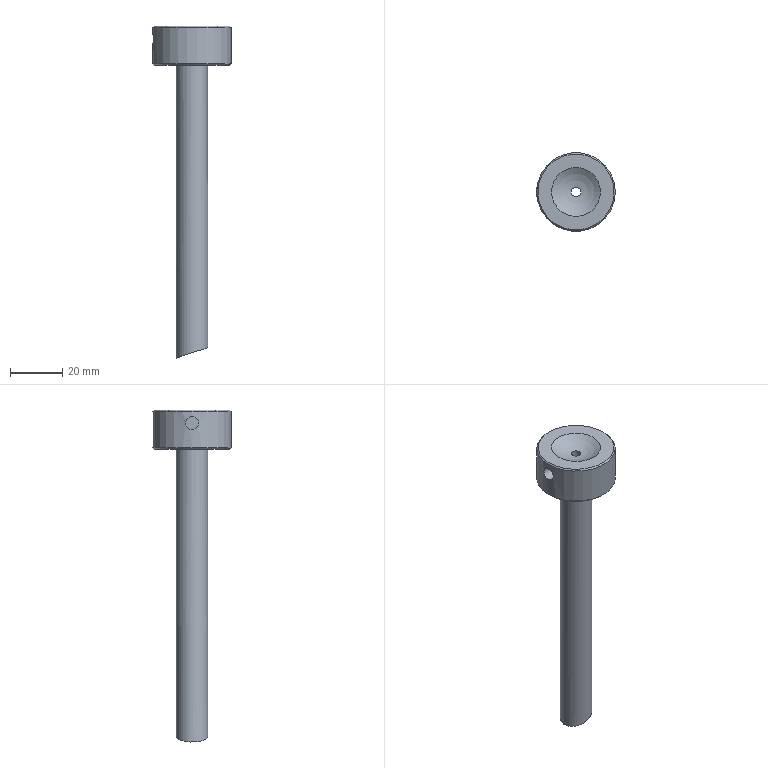Part | NX | features solid 2 | 1 solid | 11 faces | box 30 x 30 x 126.717 mm | volume 19254 mm3 | plane 3 | cylinder 3 | cone 3 | spline 1 | sphere 1 | commonest cylinder face diameters 5 x1 12 x1 30 x1
STEP:
#1=CARTESIAN_POINT('',(9.327,0.,140.5));
#2=VERTEX_POINT('',#1);
#3=CARTESIAN_POINT('',(0.,0.,140.5));
#4=DIRECTION('',(0.,0.,1.));
#5=DIRECTION('',(1.,0.,0.));
#6=AXIS2_PLACEMENT_3D('',#3,#4,#5);
#7=CIRCLE('',#6,9.327);
#8=EDGE_CURVE('',#2,#2,#7,.T.);
#9=ORIENTED_EDGE('',*,*,#8,.F.);
#10=EDGE_LOOP('',(#9));
#11=FACE_BOUND('',#10,.T.);
#12=CARTESIAN_POINT('',(14.5,0.,140.5));
#13=VERTEX_POINT('',#12);
#14=CARTESIAN_POINT('',(0.,0.,140.5));
#15=DIRECTION('',(0.,0.,1.));
#16=DIRECTION('',(1.,0.,0.));
#17=AXIS2_PLACEMENT_3D('',#14,#15,#16);
#18=CIRCLE('',#17,14.5);
#19=EDGE_CURVE('',#13,#13,#18,.T.);
#20=ORIENTED_EDGE('',*,*,#19,.T.);
#21=EDGE_LOOP('',(#20));
#22=FACE_BOUND('',#21,.T.);
#23=CARTESIAN_POINT('',(0.,0.,140.5));
#24=DIRECTION('',(0.,0.,1.));
#25=DIRECTION('',(1.,0.,0.));
#26=AXIS2_PLACEMENT_3D('',#23,#24,#25);
#27=PLANE('',#26);
#28=ADVANCED_FACE('',(#11,#22),#27,.T.);
#29=CARTESIAN_POINT('',(-6.,0.,125.5));
#30=VERTEX_POINT('',#29);
#31=CARTESIAN_POINT('',(0.,0.,125.5));
#32=DIRECTION('',(0.,0.,-1.));
#33=DIRECTION('',(-1.,0.,0.));
#34=AXIS2_PLACEMENT_3D('',#31,#32,#33);
#35=CIRCLE('',#34,6.);
#36=EDGE_CURVE('',#30,#30,#35,.T.);
#37=ORIENTED_EDGE('',*,*,#36,.F.);
#38=EDGE_LOOP('',(#37));
#39=FACE_BOUND('',#38,.T.);
#40=CARTESIAN_POINT('',(-14.5,0.,125.5));
#41=VERTEX_POINT('',#40);
#42=CARTESIAN_POINT('',(0.,0.,125.5));
#43=DIRECTION('',(0.,0.,-1.));
#44=DIRECTION('',(-1.,0.,0.));
#45=AXIS2_PLACEMENT_3D('',#42,#43,#44);
#46=CIRCLE('',#45,14.5);
#47=EDGE_CURVE('',#41,#41,#46,.T.);
#48=ORIENTED_EDGE('',*,*,#47,.T.);
#49=EDGE_LOOP('',(#48));
#50=FACE_BOUND('',#49,.T.);
#51=CARTESIAN_POINT('',(0.,0.,125.5));
#52=DIRECTION('',(0.,0.,-1.));
#53=DIRECTION('',(-1.,0.,0.));
#54=AXIS2_PLACEMENT_3D('',#51,#52,#53);
#55=PLANE('',#54);
#56=ADVANCED_FACE('',(#39,#50),#55,.T.);
#57=CARTESIAN_POINT('',(-15.,0.,138.));
#58=VERTEX_POINT('',#57);
#59=CARTESIAN_POINT('',(-14.896,-1.961,137.457));
#60=CARTESIAN_POINT('',(-15.052,0.0004642,138.271));
#61=CARTESIAN_POINT('',(-14.896,1.959,137.458));
#62=CARTESIAN_POINT('',(-14.737,2.77,135.502));
#63=CARTESIAN_POINT('',(-14.896,1.96,133.541));
#64=CARTESIAN_POINT('',(-15.052,0.0007333,132.73));
#65=CARTESIAN_POINT('',(-14.896,-1.957,133.539));
#66=CARTESIAN_POINT('',(-14.737,-2.771,135.498));
#67=CARTESIAN_POINT('',(-14.896,-1.961,137.457));
#68=CARTESIAN_POINT('',(-15.052,0.0004642,138.271));
#69=CARTESIAN_POINT('',(-14.896,1.959,137.458));
#70=B_SPLINE_CURVE_WITH_KNOTS('',3,(#59,#60,#61,#62,#63,#64,#65,#66,#67,#68,#69),.UNSPECIFIED.,.T.,.F.,(1,1,1,1,1,1,1,1,1,1,1,1,1,1,1),(-0.005872,-0.003914,-0.001957,0.,0.001957,0.003914,0.005872,0.007829,0.009786,0.01174,0.0137,0.01566,0.01761,0.01957,0.02153),.UNSPECIFIED.);
#71=EDGE_CURVE('',#58,#58,#70,.T.);
#72=ORIENTED_EDGE('',*,*,#71,.F.);
#73=EDGE_LOOP('',(#72));
#74=FACE_BOUND('',#73,.T.);
#75=CARTESIAN_POINT('',(-15.,0.,126.));
#76=VERTEX_POINT('',#75);
#77=CARTESIAN_POINT('',(0.,0.,126.));
#78=DIRECTION('',(0.,0.,-1.));
#79=DIRECTION('',(-1.,0.,0.));
#80=AXIS2_PLACEMENT_3D('',#77,#78,#79);
#81=CIRCLE('',#80,15.);
#82=EDGE_CURVE('',#76,#76,#81,.F.);
#83=ORIENTED_EDGE('',*,*,#82,.T.);
#84=EDGE_LOOP('',(#83));
#85=FACE_BOUND('',#84,.T.);
#86=CARTESIAN_POINT('',(15.,0.,140.));
#87=VERTEX_POINT('',#86);
#88=CARTESIAN_POINT('',(0.,0.,140.));
#89=DIRECTION('',(0.,0.,1.));
#90=DIRECTION('',(1.,0.,0.));
#91=AXIS2_PLACEMENT_3D('',#88,#89,#90);
#92=CIRCLE('',#91,15.);
#93=EDGE_CURVE('',#87,#87,#92,.F.);
#94=ORIENTED_EDGE('',*,*,#93,.T.);
#95=EDGE_LOOP('',(#94));
#96=FACE_BOUND('',#95,.T.);
#97=CARTESIAN_POINT('',(0.,0.,125.5));
#98=DIRECTION('',(0.,0.,1.));
#99=DIRECTION('',(1.,0.,0.));
#100=AXIS2_PLACEMENT_3D('',#97,#98,#99);
#101=CYLINDRICAL_SURFACE('',#100,15.);
#102=ADVANCED_FACE('',(#74,#85,#96),#101,.T.);
#103=ORIENTED_EDGE('',*,*,#47,.F.);
#104=EDGE_LOOP('',(#103));
#105=FACE_BOUND('',#104,.T.);
#106=ORIENTED_EDGE('',*,*,#82,.F.);
#107=EDGE_LOOP('',(#106));
#108=FACE_BOUND('',#107,.T.);
#109=CARTESIAN_POINT('',(0.,0.,126.));
#110=DIRECTION('',(0.,0.,1.));
#111=DIRECTION('',(1.,0.,0.));
#112=AXIS2_PLACEMENT_3D('',#109,#110,#111);
#113=CONICAL_SURFACE('',#112,15.,0.7854);
#114=ADVANCED_FACE('',(#105,#108),#113,.T.);
#115=ORIENTED_EDGE('',*,*,#19,.F.);
#116=EDGE_LOOP('',(#115));
#117=FACE_BOUND('',#116,.T.);
#118=ORIENTED_EDGE('',*,*,#93,.F.);
#119=EDGE_LOOP('',(#118));
#120=FACE_BOUND('',#119,.T.);
#121=CARTESIAN_POINT('',(0.,0.,140.));
#122=DIRECTION('',(0.,0.,-1.));
#123=DIRECTION('',(-1.,0.,0.));
#124=AXIS2_PLACEMENT_3D('',#121,#122,#123);
#125=CONICAL_SURFACE('',#124,15.,0.7854);
#126=ADVANCED_FACE('',(#117,#120),#125,.T.);
#127=CARTESIAN_POINT('',(-3.104,2.346,14.831));
#128=VERTEX_POINT('',#127);
#129=CARTESIAN_POINT('',(-4.293,-0.6648,14.409));
#130=CARTESIAN_POINT('',(-3.424,2.631,14.724));
#131=CARTESIAN_POINT('',(-0.6353,4.217,15.682));
#132=CARTESIAN_POINT('',(2.463,3.492,16.658));
#133=CARTESIAN_POINT('',(4.249,0.663,17.182));
#134=CARTESIAN_POINT('',(3.386,-2.632,16.932));
#135=CARTESIAN_POINT('',(0.5623,-4.224,16.069));
#136=CARTESIAN_POINT('',(-2.512,-3.48,15.046));
#137=CARTESIAN_POINT('',(-4.293,-0.6648,14.409));
#138=CARTESIAN_POINT('',(-3.424,2.631,14.724));
#139=CARTESIAN_POINT('',(-0.6353,4.217,15.682));
#140=B_SPLINE_CURVE_WITH_KNOTS('',3,(#129,#130,#131,#132,#133,#134,#135,#136,#137,#138,#139),.UNSPECIFIED.,.T.,.F.,(1,1,1,1,1,1,1,1,1,1,1,1,1,1,1),(-0.009313,-0.006208,-0.003104,0.,0.003104,0.006208,0.009313,0.01242,0.01552,0.01863,0.02173,0.02483,0.02794,0.03104,0.03415),.UNSPECIFIED.);
#141=EDGE_CURVE('',#128,#128,#140,.T.);
#142=ORIENTED_EDGE('',*,*,#141,.F.);
#143=EDGE_LOOP('',(#142));
#144=FACE_BOUND('',#143,.T.);
#145=CARTESIAN_POINT('',(-5.973,0.5729,13.792));
#146=VERTEX_POINT('',#145);
#147=CARTESIAN_POINT('',(-4.144,5.179,14.485));
#148=CARTESIAN_POINT('',(-6.663,0.6502,13.528));
#149=CARTESIAN_POINT('',(-5.039,-4.342,14.153));
#150=CARTESIAN_POINT('',(-0.6317,-6.572,15.703));
#151=CARTESIAN_POINT('',(4.133,-5.207,17.166));
#152=CARTESIAN_POINT('',(6.662,-0.6502,17.866));
#153=CARTESIAN_POINT('',(5.051,4.35,17.426));
#154=CARTESIAN_POINT('',(0.5479,6.585,16.084));
#155=CARTESIAN_POINT('',(-4.144,5.179,14.485));
#156=CARTESIAN_POINT('',(-6.663,0.6502,13.528));
#157=CARTESIAN_POINT('',(-5.039,-4.342,14.153));
#158=B_SPLINE_CURVE_WITH_KNOTS('',3,(#147,#148,#149,#150,#151,#152,#153,#154,#155,#156,#157),.UNSPECIFIED.,.T.,.F.,(1,1,1,1,1,1,1,1,1,1,1,1,1,1,1),(-0.01444,-0.009626,-0.004813,0.,0.004813,0.009626,0.01444,0.01925,0.02407,0.02888,0.03369,0.0385,0.04332,0.04813,0.05294),.UNSPECIFIED.);
#159=EDGE_CURVE('',#146,#146,#158,.T.);
#160=ORIENTED_EDGE('',*,*,#159,.F.);
#161=EDGE_LOOP('',(#160));
#162=FACE_BOUND('',#161,.T.);
#163=CARTESIAN_POINT('',(-6.105,6.11,13.742));
#164=CARTESIAN_POINT('',(-6.105,-6.095,13.742));
#165=CARTESIAN_POINT('',(-2.088,6.11,15.255));
#166=CARTESIAN_POINT('',(-2.088,-6.095,15.255));
#167=CARTESIAN_POINT('',(1.987,6.11,16.562));
#168=CARTESIAN_POINT('',(1.987,-6.095,16.562));
#169=CARTESIAN_POINT('',(6.109,6.11,17.714));
#170=CARTESIAN_POINT('',(6.109,-6.095,17.714));
#171=B_SPLINE_SURFACE_WITH_KNOTS('',3,1,((#163,#164),(#165,#166),(#167,#168),(#169,#170)),.SURF_OF_LINEAR_EXTRUSION.,.F.,.F.,.F.,(4,4),(2,2),(0.6579,0.7302),(0.,1.),.PIECEWISE_BEZIER_KNOTS.);
#172=ADVANCED_FACE('',(#144,#162),#171,.T.);
#173=ORIENTED_EDGE('',*,*,#159,.T.);
#174=EDGE_LOOP('',(#173));
#175=FACE_BOUND('',#174,.T.);
#176=ORIENTED_EDGE('',*,*,#36,.T.);
#177=EDGE_LOOP('',(#176));
#178=FACE_BOUND('',#177,.T.);
#179=CARTESIAN_POINT('',(0.,0.,125.5));
#180=DIRECTION('',(0.,0.,-1.));
#181=DIRECTION('',(1.,0.,0.));
#182=AXIS2_PLACEMENT_3D('',#179,#180,#181);
#183=CYLINDRICAL_SURFACE('',#182,6.);
#184=ADVANCED_FACE('',(#175,#178),#183,.T.);
#185=CARTESIAN_POINT('',(1.748,0.,137.596));
#186=VERTEX_POINT('',#185);
#187=CARTESIAN_POINT('',(0.,0.,137.596));
#188=DIRECTION('',(0.,0.,1.));
#189=DIRECTION('',(1.,0.,0.));
#190=AXIS2_PLACEMENT_3D('',#187,#188,#189);
#191=CIRCLE('',#190,1.748);
#192=EDGE_CURVE('',#186,#186,#191,.T.);
#193=ORIENTED_EDGE('',*,*,#192,.T.);
#194=EDGE_LOOP('',(#193));
#195=FACE_BOUND('',#194,.T.);
#196=ORIENTED_EDGE('',*,*,#141,.T.);
#197=EDGE_LOOP('',(#196));
#198=FACE_BOUND('',#197,.T.);
#199=CARTESIAN_POINT('',(0.,0.,137.5));
#200=DIRECTION('',(0.,0.,-1.));
#201=DIRECTION('',(1.,0.,0.));
#202=AXIS2_PLACEMENT_3D('',#199,#200,#201);
#203=CONICAL_SURFACE('',#202,1.75,0.01745);
#204=ADVANCED_FACE('',(#195,#198),#203,.F.);
#205=ORIENTED_EDGE('',*,*,#8,.T.);
#206=EDGE_LOOP('',(#205));
#207=FACE_BOUND('',#206,.T.);
#208=ORIENTED_EDGE('',*,*,#192,.F.);
#209=EDGE_LOOP('',(#208));
#210=FACE_BOUND('',#209,.T.);
#211=CARTESIAN_POINT('',(0.,0.,153.5));
#212=DIRECTION('',(0.,0.,1.));
#213=DIRECTION('',(1.,0.,0.));
#214=AXIS2_PLACEMENT_3D('',#211,#212,#213);
#215=SPHERICAL_SURFACE('',#214,16.);
#216=ADVANCED_FACE('',(#207,#210),#215,.F.);
#217=CARTESIAN_POINT('',(-8.,0.,138.));
#218=VERTEX_POINT('',#217);
#219=CARTESIAN_POINT('',(-8.,0.,135.5));
#220=DIRECTION('',(-1.,0.,0.));
#221=DIRECTION('',(0.,0.,1.));
#222=AXIS2_PLACEMENT_3D('',#219,#220,#221);
#223=CIRCLE('',#222,2.5);
#224=EDGE_CURVE('',#218,#218,#223,.F.);
#225=ORIENTED_EDGE('',*,*,#224,.F.);
#226=EDGE_LOOP('',(#225));
#227=FACE_BOUND('',#226,.T.);
#228=CARTESIAN_POINT('',(-8.,0.,135.5));
#229=DIRECTION('',(1.,0.,0.));
#230=DIRECTION('',(0.,1.,0.));
#231=AXIS2_PLACEMENT_3D('',#228,#229,#230);
#232=PLANE('',#231);
#233=ADVANCED_FACE('',(#227),#232,.F.);
#234=ORIENTED_EDGE('',*,*,#71,.T.);
#235=EDGE_LOOP('',(#234));
#236=FACE_BOUND('',#235,.T.);
#237=ORIENTED_EDGE('',*,*,#224,.T.);
#238=EDGE_LOOP('',(#237));
#239=FACE_BOUND('',#238,.T.);
#240=CARTESIAN_POINT('',(-8.,0.,135.5));
#241=DIRECTION('',(-1.,0.,0.));
#242=DIRECTION('',(0.,0.,1.));
#243=AXIS2_PLACEMENT_3D('',#240,#241,#242);
#244=CYLINDRICAL_SURFACE('',#243,2.5);
#245=ADVANCED_FACE('',(#236,#239),#244,.F.);
#246=CLOSED_SHELL('',(#28,#56,#102,#114,#126,#172,#184,#204,#216,#233,#245));
#247=MANIFOLD_SOLID_BREP('',#246);
#248=(LENGTH_UNIT()NAMED_UNIT(*)SI_UNIT(.MILLI.,.METRE.));
#249=UNCERTAINTY_MEASURE_WITH_UNIT(LENGTH_MEASURE(0.0508),#248,'','');
#250=(NAMED_UNIT(*)PLANE_ANGLE_UNIT()SI_UNIT($,.RADIAN.));
#251=(NAMED_UNIT(*)SI_UNIT($,.STERADIAN.)SOLID_ANGLE_UNIT());
#252=(GEOMETRIC_REPRESENTATION_CONTEXT(3)GLOBAL_UNCERTAINTY_ASSIGNED_CONTEXT((#249))GLOBAL_UNIT_ASSIGNED_CONTEXT((#248,#250,#251))REPRESENTATION_CONTEXT('',''));
#253=ADVANCED_BREP_SHAPE_REPRESENTATION('',(#247),#252);